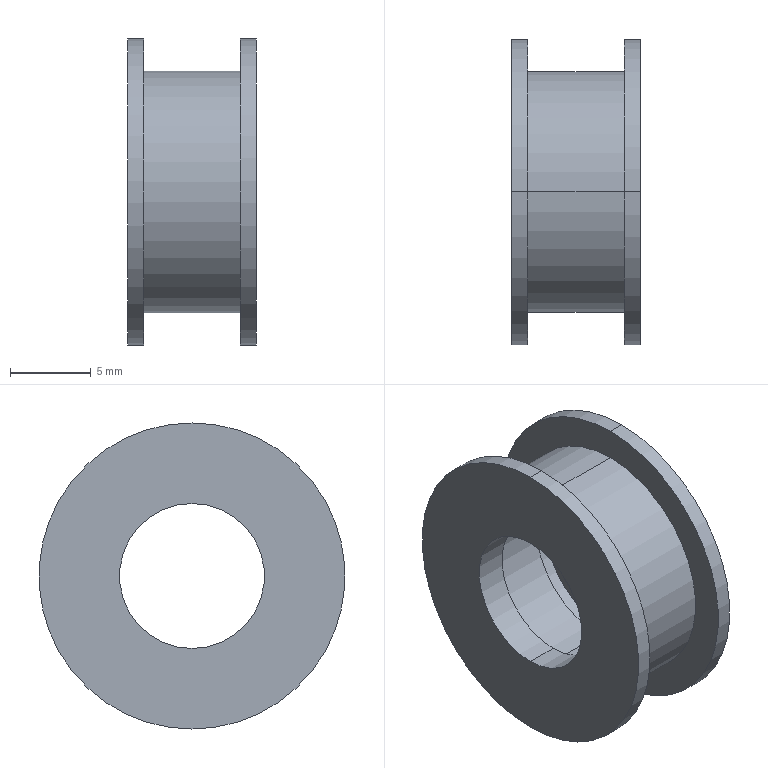Part | SolidWorks | features RefAxis 12, 3DProfileFeature 4, Revolution 1 | 1 solid | 21 faces | box 8 x 19 x 19 mm | volume 915.586 mm3 | cylinder 14 | plane 7 | commonest cylinder face diameters 11 x4 19 x4 9 x2 11.8 x2 15 x2
STEP:
#1=CARTESIAN_POINT('',(-3.,0.,9.5));
#2=VERTEX_POINT('',#1);
#3=CARTESIAN_POINT('',(-3.,0.,-9.5));
#4=VERTEX_POINT('',#3);
#5=CARTESIAN_POINT('',(-3.,0.,0.));
#6=DIRECTION('',(-1.,0.,0.));
#7=DIRECTION('',(0.,0.,1.));
#8=AXIS2_PLACEMENT_3D('',#5,#6,#7);
#9=CIRCLE('',#8,9.5);
#10=EDGE_CURVE('',#2,#4,#9,.T.);
#11=ORIENTED_EDGE('',*,*,#10,.T.);
#12=CARTESIAN_POINT('',(-4.,0.,-9.5));
#13=VERTEX_POINT('',#12);
#14=CARTESIAN_POINT('',(4.,0.,-9.5));
#15=DIRECTION('',(-1.,0.,0.));
#16=VECTOR('',#15,1000.);
#17=LINE('',#14,#16);
#18=EDGE_CURVE('',#4,#13,#17,.T.);
#19=ORIENTED_EDGE('',*,*,#18,.T.);
#20=CARTESIAN_POINT('',(-4.,0.,9.5));
#21=VERTEX_POINT('',#20);
#22=CARTESIAN_POINT('',(-4.,0.,0.));
#23=DIRECTION('',(-1.,0.,0.));
#24=DIRECTION('',(0.,0.,1.));
#25=AXIS2_PLACEMENT_3D('',#22,#23,#24);
#26=CIRCLE('',#25,9.5);
#27=EDGE_CURVE('',#21,#13,#26,.T.);
#28=ORIENTED_EDGE('',*,*,#27,.F.);
#29=CARTESIAN_POINT('',(4.,0.,9.5));
#30=DIRECTION('',(-1.,0.,0.));
#31=VECTOR('',#30,1000.);
#32=LINE('',#29,#31);
#33=EDGE_CURVE('',#2,#21,#32,.T.);
#34=ORIENTED_EDGE('',*,*,#33,.F.);
#35=EDGE_LOOP('',(#11,#19,#28,#34));
#36=FACE_OUTER_BOUND('',#35,.T.);
#37=CARTESIAN_POINT('',(4.,0.,0.));
#38=DIRECTION('',(-1.,0.,0.));
#39=DIRECTION('',(0.,0.,1.));
#40=AXIS2_PLACEMENT_3D('',#37,#38,#39);
#41=CYLINDRICAL_SURFACE('',#40,9.5);
#42=ADVANCED_FACE('',(#36),#41,.T.);
#43=CARTESIAN_POINT('',(3.,0.,7.5));
#44=VERTEX_POINT('',#43);
#45=CARTESIAN_POINT('',(3.,0.,-7.5));
#46=VERTEX_POINT('',#45);
#47=CARTESIAN_POINT('',(3.,0.,0.));
#48=DIRECTION('',(-1.,0.,0.));
#49=DIRECTION('',(0.,0.,1.));
#50=AXIS2_PLACEMENT_3D('',#47,#48,#49);
#51=CIRCLE('',#50,7.5);
#52=EDGE_CURVE('',#44,#46,#51,.T.);
#53=ORIENTED_EDGE('',*,*,#52,.T.);
#54=CARTESIAN_POINT('',(-3.,0.,-7.5));
#55=VERTEX_POINT('',#54);
#56=CARTESIAN_POINT('',(4.,0.,-7.5));
#57=DIRECTION('',(-1.,0.,0.));
#58=VECTOR('',#57,1000.);
#59=LINE('',#56,#58);
#60=EDGE_CURVE('',#46,#55,#59,.T.);
#61=ORIENTED_EDGE('',*,*,#60,.T.);
#62=CARTESIAN_POINT('',(-3.,0.,7.5));
#63=VERTEX_POINT('',#62);
#64=CARTESIAN_POINT('',(-3.,0.,0.));
#65=DIRECTION('',(-1.,0.,0.));
#66=DIRECTION('',(0.,0.,1.));
#67=AXIS2_PLACEMENT_3D('',#64,#65,#66);
#68=CIRCLE('',#67,7.5);
#69=EDGE_CURVE('',#63,#55,#68,.T.);
#70=ORIENTED_EDGE('',*,*,#69,.F.);
#71=CARTESIAN_POINT('',(4.,0.,7.5));
#72=DIRECTION('',(-1.,0.,0.));
#73=VECTOR('',#72,1000.);
#74=LINE('',#71,#73);
#75=EDGE_CURVE('',#44,#63,#74,.T.);
#76=ORIENTED_EDGE('',*,*,#75,.F.);
#77=EDGE_LOOP('',(#53,#61,#70,#76));
#78=FACE_OUTER_BOUND('',#77,.T.);
#79=CARTESIAN_POINT('',(4.,0.,0.));
#80=DIRECTION('',(-1.,0.,0.));
#81=DIRECTION('',(0.,0.,1.));
#82=AXIS2_PLACEMENT_3D('',#79,#80,#81);
#83=CYLINDRICAL_SURFACE('',#82,7.5);
#84=ADVANCED_FACE('',(#78),#83,.T.);
#85=CARTESIAN_POINT('',(4.,0.,9.5));
#86=VERTEX_POINT('',#85);
#87=CARTESIAN_POINT('',(4.,0.,-9.5));
#88=VERTEX_POINT('',#87);
#89=CARTESIAN_POINT('',(4.,0.,0.));
#90=DIRECTION('',(-1.,0.,0.));
#91=DIRECTION('',(0.,0.,1.));
#92=AXIS2_PLACEMENT_3D('',#89,#90,#91);
#93=CIRCLE('',#92,9.5);
#94=EDGE_CURVE('',#86,#88,#93,.T.);
#95=ORIENTED_EDGE('',*,*,#94,.T.);
#96=CARTESIAN_POINT('',(3.,0.,-9.5));
#97=VERTEX_POINT('',#96);
#98=CARTESIAN_POINT('',(4.,0.,-9.5));
#99=DIRECTION('',(-1.,0.,0.));
#100=VECTOR('',#99,1000.);
#101=LINE('',#98,#100);
#102=EDGE_CURVE('',#88,#97,#101,.T.);
#103=ORIENTED_EDGE('',*,*,#102,.T.);
#104=CARTESIAN_POINT('',(3.,0.,9.5));
#105=VERTEX_POINT('',#104);
#106=CARTESIAN_POINT('',(3.,0.,0.));
#107=DIRECTION('',(-1.,0.,0.));
#108=DIRECTION('',(0.,0.,1.));
#109=AXIS2_PLACEMENT_3D('',#106,#107,#108);
#110=CIRCLE('',#109,9.5);
#111=EDGE_CURVE('',#105,#97,#110,.T.);
#112=ORIENTED_EDGE('',*,*,#111,.F.);
#113=CARTESIAN_POINT('',(4.,0.,9.5));
#114=DIRECTION('',(-1.,0.,0.));
#115=VECTOR('',#114,1000.);
#116=LINE('',#113,#115);
#117=EDGE_CURVE('',#86,#105,#116,.T.);
#118=ORIENTED_EDGE('',*,*,#117,.F.);
#119=EDGE_LOOP('',(#95,#103,#112,#118));
#120=FACE_OUTER_BOUND('',#119,.T.);
#121=CARTESIAN_POINT('',(4.,0.,0.));
#122=DIRECTION('',(-1.,0.,0.));
#123=DIRECTION('',(0.,0.,1.));
#124=AXIS2_PLACEMENT_3D('',#121,#122,#123);
#125=CYLINDRICAL_SURFACE('',#124,9.5);
#126=ADVANCED_FACE('',(#120),#125,.T.);
#127=CARTESIAN_POINT('',(4.,0.,-5.5));
#128=VERTEX_POINT('',#127);
#129=CARTESIAN_POINT('',(4.,0.,5.5));
#130=VERTEX_POINT('',#129);
#131=CARTESIAN_POINT('',(4.,0.,0.));
#132=DIRECTION('',(-1.,0.,0.));
#133=DIRECTION('',(0.,0.,1.));
#134=AXIS2_PLACEMENT_3D('',#131,#132,#133);
#135=CIRCLE('',#134,5.5);
#136=EDGE_CURVE('',#128,#130,#135,.T.);
#137=ORIENTED_EDGE('',*,*,#136,.F.);
#138=CARTESIAN_POINT('',(3.,0.,-5.5));
#139=VERTEX_POINT('',#138);
#140=CARTESIAN_POINT('',(4.,0.,-5.5));
#141=DIRECTION('',(-1.,0.,0.));
#142=VECTOR('',#141,1000.);
#143=LINE('',#140,#142);
#144=EDGE_CURVE('',#128,#139,#143,.T.);
#145=ORIENTED_EDGE('',*,*,#144,.T.);
#146=CARTESIAN_POINT('',(3.,0.,5.5));
#147=VERTEX_POINT('',#146);
#148=CARTESIAN_POINT('',(3.,0.,0.));
#149=DIRECTION('',(-1.,0.,0.));
#150=DIRECTION('',(0.,0.,1.));
#151=AXIS2_PLACEMENT_3D('',#148,#149,#150);
#152=CIRCLE('',#151,5.5);
#153=EDGE_CURVE('',#139,#147,#152,.T.);
#154=ORIENTED_EDGE('',*,*,#153,.T.);
#155=CARTESIAN_POINT('',(4.,0.,5.5));
#156=DIRECTION('',(-1.,0.,0.));
#157=VECTOR('',#156,1000.);
#158=LINE('',#155,#157);
#159=EDGE_CURVE('',#130,#147,#158,.T.);
#160=ORIENTED_EDGE('',*,*,#159,.F.);
#161=EDGE_LOOP('',(#137,#145,#154,#160));
#162=FACE_OUTER_BOUND('',#161,.T.);
#163=CARTESIAN_POINT('',(4.,0.,0.));
#164=DIRECTION('',(-1.,0.,0.));
#165=DIRECTION('',(0.,0.,1.));
#166=AXIS2_PLACEMENT_3D('',#163,#164,#165);
#167=CYLINDRICAL_SURFACE('',#166,5.5);
#168=ADVANCED_FACE('',(#162),#167,.F.);
#169=CARTESIAN_POINT('',(3.,0.,-5.9));
#170=VERTEX_POINT('',#169);
#171=CARTESIAN_POINT('',(3.,0.,5.9));
#172=VERTEX_POINT('',#171);
#173=CARTESIAN_POINT('',(3.,0.,0.));
#174=DIRECTION('',(-1.,0.,0.));
#175=DIRECTION('',(0.,0.,1.));
#176=AXIS2_PLACEMENT_3D('',#173,#174,#175);
#177=CIRCLE('',#176,5.9);
#178=EDGE_CURVE('',#170,#172,#177,.T.);
#179=ORIENTED_EDGE('',*,*,#178,.F.);
#180=CARTESIAN_POINT('',(2.,0.,-5.9));
#181=VERTEX_POINT('',#180);
#182=CARTESIAN_POINT('',(4.,0.,-5.9));
#183=DIRECTION('',(-1.,0.,0.));
#184=VECTOR('',#183,1000.);
#185=LINE('',#182,#184);
#186=EDGE_CURVE('',#170,#181,#185,.T.);
#187=ORIENTED_EDGE('',*,*,#186,.T.);
#188=CARTESIAN_POINT('',(2.,0.,5.9));
#189=VERTEX_POINT('',#188);
#190=CARTESIAN_POINT('',(2.,0.,0.));
#191=DIRECTION('',(-1.,0.,0.));
#192=DIRECTION('',(0.,0.,1.));
#193=AXIS2_PLACEMENT_3D('',#190,#191,#192);
#194=CIRCLE('',#193,5.9);
#195=EDGE_CURVE('',#181,#189,#194,.T.);
#196=ORIENTED_EDGE('',*,*,#195,.T.);
#197=CARTESIAN_POINT('',(4.,0.,5.9));
#198=DIRECTION('',(-1.,0.,0.));
#199=VECTOR('',#198,1000.);
#200=LINE('',#197,#199);
#201=EDGE_CURVE('',#172,#189,#200,.T.);
#202=ORIENTED_EDGE('',*,*,#201,.F.);
#203=EDGE_LOOP('',(#179,#187,#196,#202));
#204=FACE_OUTER_BOUND('',#203,.T.);
#205=CARTESIAN_POINT('',(4.,0.,0.));
#206=DIRECTION('',(-1.,0.,0.));
#207=DIRECTION('',(0.,0.,1.));
#208=AXIS2_PLACEMENT_3D('',#205,#206,#207);
#209=CYLINDRICAL_SURFACE('',#208,5.9);
#210=ADVANCED_FACE('',(#204),#209,.F.);
#211=CARTESIAN_POINT('',(2.,0.,-5.5));
#212=VERTEX_POINT('',#211);
#213=CARTESIAN_POINT('',(2.,0.,5.5));
#214=VERTEX_POINT('',#213);
#215=CARTESIAN_POINT('',(2.,0.,0.));
#216=DIRECTION('',(-1.,0.,0.));
#217=DIRECTION('',(0.,0.,1.));
#218=AXIS2_PLACEMENT_3D('',#215,#216,#217);
#219=CIRCLE('',#218,5.5);
#220=EDGE_CURVE('',#212,#214,#219,.T.);
#221=ORIENTED_EDGE('',*,*,#220,.F.);
#222=CARTESIAN_POINT('',(-2.,0.,-5.5));
#223=VERTEX_POINT('',#222);
#224=CARTESIAN_POINT('',(4.,0.,-5.5));
#225=DIRECTION('',(-1.,0.,0.));
#226=VECTOR('',#225,1000.);
#227=LINE('',#224,#226);
#228=EDGE_CURVE('',#212,#223,#227,.T.);
#229=ORIENTED_EDGE('',*,*,#228,.T.);
#230=CARTESIAN_POINT('',(-2.,0.,5.5));
#231=VERTEX_POINT('',#230);
#232=CARTESIAN_POINT('',(-2.,0.,0.));
#233=DIRECTION('',(-1.,0.,0.));
#234=DIRECTION('',(0.,0.,1.));
#235=AXIS2_PLACEMENT_3D('',#232,#233,#234);
#236=CIRCLE('',#235,5.5);
#237=EDGE_CURVE('',#223,#231,#236,.T.);
#238=ORIENTED_EDGE('',*,*,#237,.T.);
#239=CARTESIAN_POINT('',(4.,0.,5.5));
#240=DIRECTION('',(-1.,0.,0.));
#241=VECTOR('',#240,1000.);
#242=LINE('',#239,#241);
#243=EDGE_CURVE('',#214,#231,#242,.T.);
#244=ORIENTED_EDGE('',*,*,#243,.F.);
#245=EDGE_LOOP('',(#221,#229,#238,#244));
#246=FACE_OUTER_BOUND('',#245,.T.);
#247=CARTESIAN_POINT('',(4.,0.,0.));
#248=DIRECTION('',(-1.,0.,0.));
#249=DIRECTION('',(0.,0.,1.));
#250=AXIS2_PLACEMENT_3D('',#247,#248,#249);
#251=CYLINDRICAL_SURFACE('',#250,5.5);
#252=ADVANCED_FACE('',(#246),#251,.F.);
#253=CARTESIAN_POINT('',(-2.,0.,-4.5));
#254=VERTEX_POINT('',#253);
#255=CARTESIAN_POINT('',(-2.,0.,4.5));
#256=VERTEX_POINT('',#255);
#257=CARTESIAN_POINT('',(-2.,0.,0.));
#258=DIRECTION('',(-1.,0.,0.));
#259=DIRECTION('',(0.,0.,1.));
#260=AXIS2_PLACEMENT_3D('',#257,#258,#259);
#261=CIRCLE('',#260,4.5);
#262=EDGE_CURVE('',#254,#256,#261,.T.);
#263=ORIENTED_EDGE('',*,*,#262,.F.);
#264=CARTESIAN_POINT('',(-4.,0.,-4.5));
#265=VERTEX_POINT('',#264);
#266=CARTESIAN_POINT('',(4.,0.,-4.5));
#267=DIRECTION('',(-1.,0.,0.));
#268=VECTOR('',#267,1000.);
#269=LINE('',#266,#268);
#270=EDGE_CURVE('',#254,#265,#269,.T.);
#271=ORIENTED_EDGE('',*,*,#270,.T.);
#272=CARTESIAN_POINT('',(-4.,0.,4.5));
#273=VERTEX_POINT('',#272);
#274=CARTESIAN_POINT('',(-4.,0.,0.));
#275=DIRECTION('',(-1.,0.,0.));
#276=DIRECTION('',(0.,0.,1.));
#277=AXIS2_PLACEMENT_3D('',#274,#275,#276);
#278=CIRCLE('',#277,4.5);
#279=EDGE_CURVE('',#265,#273,#278,.T.);
#280=ORIENTED_EDGE('',*,*,#279,.T.);
#281=CARTESIAN_POINT('',(4.,0.,4.5));
#282=DIRECTION('',(-1.,0.,0.));
#283=VECTOR('',#282,1000.);
#284=LINE('',#281,#283);
#285=EDGE_CURVE('',#256,#273,#284,.T.);
#286=ORIENTED_EDGE('',*,*,#285,.F.);
#287=EDGE_LOOP('',(#263,#271,#280,#286));
#288=FACE_OUTER_BOUND('',#287,.T.);
#289=CARTESIAN_POINT('',(4.,0.,0.));
#290=DIRECTION('',(-1.,0.,0.));
#291=DIRECTION('',(0.,0.,1.));
#292=AXIS2_PLACEMENT_3D('',#289,#290,#291);
#293=CYLINDRICAL_SURFACE('',#292,4.5);
#294=ADVANCED_FACE('',(#288),#293,.F.);
#295=CARTESIAN_POINT('',(-4.,0.,0.));
#296=DIRECTION('',(-1.,0.,0.));
#297=DIRECTION('',(0.,0.,1.));
#298=AXIS2_PLACEMENT_3D('',#295,#296,#297);
#299=CIRCLE('',#298,4.5);
#300=EDGE_CURVE('',#273,#265,#299,.T.);
#301=ORIENTED_EDGE('',*,*,#300,.F.);
#302=ORIENTED_EDGE('',*,*,#279,.F.);
#303=EDGE_LOOP('',(#301,#302));
#304=FACE_BOUND('',#303,.T.);
#305=ORIENTED_EDGE('',*,*,#27,.T.);
#306=CARTESIAN_POINT('',(-4.,0.,0.));
#307=DIRECTION('',(-1.,0.,0.));
#308=DIRECTION('',(0.,0.,1.));
#309=AXIS2_PLACEMENT_3D('',#306,#307,#308);
#310=CIRCLE('',#309,9.5);
#311=EDGE_CURVE('',#13,#21,#310,.T.);
#312=ORIENTED_EDGE('',*,*,#311,.T.);
#313=EDGE_LOOP('',(#305,#312));
#314=FACE_OUTER_BOUND('',#313,.T.);
#315=CARTESIAN_POINT('',(-4.,9.5,0.));
#316=DIRECTION('',(1.,0.,0.));
#317=DIRECTION('',(0.,0.,-1.));
#318=AXIS2_PLACEMENT_3D('',#315,#316,#317);
#319=PLANE('',#318);
#320=ADVANCED_FACE('',(#304,#314),#319,.F.);
#321=ORIENTED_EDGE('',*,*,#270,.F.);
#322=CARTESIAN_POINT('',(-2.,0.,0.));
#323=DIRECTION('',(-1.,0.,0.));
#324=DIRECTION('',(0.,0.,1.));
#325=AXIS2_PLACEMENT_3D('',#322,#323,#324);
#326=CIRCLE('',#325,4.5);
#327=EDGE_CURVE('',#256,#254,#326,.T.);
#328=ORIENTED_EDGE('',*,*,#327,.F.);
#329=ORIENTED_EDGE('',*,*,#285,.T.);
#330=ORIENTED_EDGE('',*,*,#300,.T.);
#331=EDGE_LOOP('',(#321,#328,#329,#330));
#332=FACE_OUTER_BOUND('',#331,.T.);
#333=CARTESIAN_POINT('',(4.,0.,0.));
#334=DIRECTION('',(-1.,0.,0.));
#335=DIRECTION('',(0.,0.,1.));
#336=AXIS2_PLACEMENT_3D('',#333,#334,#335);
#337=CYLINDRICAL_SURFACE('',#336,4.5);
#338=ADVANCED_FACE('',(#332),#337,.F.);
#339=CARTESIAN_POINT('',(-2.,0.,0.));
#340=DIRECTION('',(-1.,0.,0.));
#341=DIRECTION('',(0.,0.,1.));
#342=AXIS2_PLACEMENT_3D('',#339,#340,#341);
#343=CIRCLE('',#342,5.5);
#344=EDGE_CURVE('',#231,#223,#343,.T.);
#345=ORIENTED_EDGE('',*,*,#344,.F.);
#346=ORIENTED_EDGE('',*,*,#237,.F.);
#347=EDGE_LOOP('',(#345,#346));
#348=FACE_OUTER_BOUND('',#347,.T.);
#349=ORIENTED_EDGE('',*,*,#327,.T.);
#350=ORIENTED_EDGE('',*,*,#262,.T.);
#351=EDGE_LOOP('',(#349,#350));
#352=FACE_BOUND('',#351,.T.);
#353=CARTESIAN_POINT('',(-2.,4.5,0.));
#354=DIRECTION('',(-1.,0.,0.));
#355=DIRECTION('',(0.,0.,1.));
#356=AXIS2_PLACEMENT_3D('',#353,#354,#355);
#357=PLANE('',#356);
#358=ADVANCED_FACE('',(#348,#352),#357,.F.);
#359=ORIENTED_EDGE('',*,*,#228,.F.);
#360=CARTESIAN_POINT('',(2.,0.,0.));
#361=DIRECTION('',(-1.,0.,0.));
#362=DIRECTION('',(0.,0.,1.));
#363=AXIS2_PLACEMENT_3D('',#360,#361,#362);
#364=CIRCLE('',#363,5.5);
#365=EDGE_CURVE('',#214,#212,#364,.T.);
#366=ORIENTED_EDGE('',*,*,#365,.F.);
#367=ORIENTED_EDGE('',*,*,#243,.T.);
#368=ORIENTED_EDGE('',*,*,#344,.T.);
#369=EDGE_LOOP('',(#359,#366,#367,#368));
#370=FACE_OUTER_BOUND('',#369,.T.);
#371=CARTESIAN_POINT('',(4.,0.,0.));
#372=DIRECTION('',(-1.,0.,0.));
#373=DIRECTION('',(0.,0.,1.));
#374=AXIS2_PLACEMENT_3D('',#371,#372,#373);
#375=CYLINDRICAL_SURFACE('',#374,5.5);
#376=ADVANCED_FACE('',(#370),#375,.F.);
#377=CARTESIAN_POINT('',(2.,0.,0.));
#378=DIRECTION('',(-1.,0.,0.));
#379=DIRECTION('',(0.,0.,1.));
#380=AXIS2_PLACEMENT_3D('',#377,#378,#379);
#381=CIRCLE('',#380,5.9);
#382=EDGE_CURVE('',#189,#181,#381,.T.);
#383=ORIENTED_EDGE('',*,*,#382,.F.);
#384=ORIENTED_EDGE('',*,*,#195,.F.);
#385=EDGE_LOOP('',(#383,#384));
#386=FACE_OUTER_BOUND('',#385,.T.);
#387=ORIENTED_EDGE('',*,*,#365,.T.);
#388=ORIENTED_EDGE('',*,*,#220,.T.);
#389=EDGE_LOOP('',(#387,#388));
#390=FACE_BOUND('',#389,.T.);
#391=CARTESIAN_POINT('',(2.,5.5,0.));
#392=DIRECTION('',(-1.,0.,0.));
#393=DIRECTION('',(0.,0.,1.));
#394=AXIS2_PLACEMENT_3D('',#391,#392,#393);
#395=PLANE('',#394);
#396=ADVANCED_FACE('',(#386,#390),#395,.F.);
#397=ORIENTED_EDGE('',*,*,#186,.F.);
#398=CARTESIAN_POINT('',(3.,0.,0.));
#399=DIRECTION('',(-1.,0.,0.));
#400=DIRECTION('',(0.,0.,1.));
#401=AXIS2_PLACEMENT_3D('',#398,#399,#400);
#402=CIRCLE('',#401,5.9);
#403=EDGE_CURVE('',#172,#170,#402,.T.);
#404=ORIENTED_EDGE('',*,*,#403,.F.);
#405=ORIENTED_EDGE('',*,*,#201,.T.);
#406=ORIENTED_EDGE('',*,*,#382,.T.);
#407=EDGE_LOOP('',(#397,#404,#405,#406));
#408=FACE_OUTER_BOUND('',#407,.T.);
#409=CARTESIAN_POINT('',(4.,0.,0.));
#410=DIRECTION('',(-1.,0.,0.));
#411=DIRECTION('',(0.,0.,1.));
#412=AXIS2_PLACEMENT_3D('',#409,#410,#411);
#413=CYLINDRICAL_SURFACE('',#412,5.9);
#414=ADVANCED_FACE('',(#408),#413,.F.);
#415=CARTESIAN_POINT('',(3.,0.,0.));
#416=DIRECTION('',(-1.,0.,0.));
#417=DIRECTION('',(0.,0.,1.));
#418=AXIS2_PLACEMENT_3D('',#415,#416,#417);
#419=CIRCLE('',#418,5.5);
#420=EDGE_CURVE('',#147,#139,#419,.T.);
#421=ORIENTED_EDGE('',*,*,#420,.F.);
#422=ORIENTED_EDGE('',*,*,#153,.F.);
#423=EDGE_LOOP('',(#421,#422));
#424=FACE_BOUND('',#423,.T.);
#425=ORIENTED_EDGE('',*,*,#403,.T.);
#426=ORIENTED_EDGE('',*,*,#178,.T.);
#427=EDGE_LOOP('',(#425,#426));
#428=FACE_OUTER_BOUND('',#427,.T.);
#429=CARTESIAN_POINT('',(3.,5.9,0.));
#430=DIRECTION('',(1.,0.,0.));
#431=DIRECTION('',(0.,0.,-1.));
#432=AXIS2_PLACEMENT_3D('',#429,#430,#431);
#433=PLANE('',#432);
#434=ADVANCED_FACE('',(#424,#428),#433,.F.);
#435=ORIENTED_EDGE('',*,*,#144,.F.);
#436=CARTESIAN_POINT('',(4.,0.,0.));
#437=DIRECTION('',(-1.,0.,0.));
#438=DIRECTION('',(0.,0.,1.));
#439=AXIS2_PLACEMENT_3D('',#436,#437,#438);
#440=CIRCLE('',#439,5.5);
#441=EDGE_CURVE('',#130,#128,#440,.T.);
#442=ORIENTED_EDGE('',*,*,#441,.F.);
#443=ORIENTED_EDGE('',*,*,#159,.T.);
#444=ORIENTED_EDGE('',*,*,#420,.T.);
#445=EDGE_LOOP('',(#435,#442,#443,#444));
#446=FACE_OUTER_BOUND('',#445,.T.);
#447=CARTESIAN_POINT('',(4.,0.,0.));
#448=DIRECTION('',(-1.,0.,0.));
#449=DIRECTION('',(0.,0.,1.));
#450=AXIS2_PLACEMENT_3D('',#447,#448,#449);
#451=CYLINDRICAL_SURFACE('',#450,5.5);
#452=ADVANCED_FACE('',(#446),#451,.F.);
#453=ORIENTED_EDGE('',*,*,#94,.F.);
#454=CARTESIAN_POINT('',(4.,0.,0.));
#455=DIRECTION('',(-1.,0.,0.));
#456=DIRECTION('',(0.,0.,1.));
#457=AXIS2_PLACEMENT_3D('',#454,#455,#456);
#458=CIRCLE('',#457,9.5);
#459=EDGE_CURVE('',#88,#86,#458,.T.);
#460=ORIENTED_EDGE('',*,*,#459,.F.);
#461=EDGE_LOOP('',(#453,#460));
#462=FACE_OUTER_BOUND('',#461,.T.);
#463=ORIENTED_EDGE('',*,*,#441,.T.);
#464=ORIENTED_EDGE('',*,*,#136,.T.);
#465=EDGE_LOOP('',(#463,#464));
#466=FACE_BOUND('',#465,.T.);
#467=CARTESIAN_POINT('',(4.,5.5,0.));
#468=DIRECTION('',(-1.,0.,0.));
#469=DIRECTION('',(0.,0.,1.));
#470=AXIS2_PLACEMENT_3D('',#467,#468,#469);
#471=PLANE('',#470);
#472=ADVANCED_FACE('',(#462,#466),#471,.F.);
#473=ORIENTED_EDGE('',*,*,#102,.F.);
#474=ORIENTED_EDGE('',*,*,#459,.T.);
#475=ORIENTED_EDGE('',*,*,#117,.T.);
#476=CARTESIAN_POINT('',(3.,0.,0.));
#477=DIRECTION('',(-1.,0.,0.));
#478=DIRECTION('',(0.,0.,1.));
#479=AXIS2_PLACEMENT_3D('',#476,#477,#478);
#480=CIRCLE('',#479,9.5);
#481=EDGE_CURVE('',#97,#105,#480,.T.);
#482=ORIENTED_EDGE('',*,*,#481,.F.);
#483=EDGE_LOOP('',(#473,#474,#475,#482));
#484=FACE_OUTER_BOUND('',#483,.T.);
#485=CARTESIAN_POINT('',(4.,0.,0.));
#486=DIRECTION('',(-1.,0.,0.));
#487=DIRECTION('',(0.,0.,1.));
#488=AXIS2_PLACEMENT_3D('',#485,#486,#487);
#489=CYLINDRICAL_SURFACE('',#488,9.5);
#490=ADVANCED_FACE('',(#484),#489,.T.);
#491=ORIENTED_EDGE('',*,*,#52,.F.);
#492=CARTESIAN_POINT('',(3.,0.,0.));
#493=DIRECTION('',(-1.,0.,0.));
#494=DIRECTION('',(0.,0.,1.));
#495=AXIS2_PLACEMENT_3D('',#492,#493,#494);
#496=CIRCLE('',#495,7.5);
#497=EDGE_CURVE('',#46,#44,#496,.T.);
#498=ORIENTED_EDGE('',*,*,#497,.F.);
#499=EDGE_LOOP('',(#491,#498));
#500=FACE_BOUND('',#499,.T.);
#501=ORIENTED_EDGE('',*,*,#111,.T.);
#502=ORIENTED_EDGE('',*,*,#481,.T.);
#503=EDGE_LOOP('',(#501,#502));
#504=FACE_OUTER_BOUND('',#503,.T.);
#505=CARTESIAN_POINT('',(3.,9.5,0.));
#506=DIRECTION('',(1.,0.,0.));
#507=DIRECTION('',(0.,0.,-1.));
#508=AXIS2_PLACEMENT_3D('',#505,#506,#507);
#509=PLANE('',#508);
#510=ADVANCED_FACE('',(#500,#504),#509,.F.);
#511=ORIENTED_EDGE('',*,*,#60,.F.);
#512=ORIENTED_EDGE('',*,*,#497,.T.);
#513=ORIENTED_EDGE('',*,*,#75,.T.);
#514=CARTESIAN_POINT('',(-3.,0.,0.));
#515=DIRECTION('',(-1.,0.,0.));
#516=DIRECTION('',(0.,0.,1.));
#517=AXIS2_PLACEMENT_3D('',#514,#515,#516);
#518=CIRCLE('',#517,7.5);
#519=EDGE_CURVE('',#55,#63,#518,.T.);
#520=ORIENTED_EDGE('',*,*,#519,.F.);
#521=EDGE_LOOP('',(#511,#512,#513,#520));
#522=FACE_OUTER_BOUND('',#521,.T.);
#523=CARTESIAN_POINT('',(4.,0.,0.));
#524=DIRECTION('',(-1.,0.,0.));
#525=DIRECTION('',(0.,0.,1.));
#526=AXIS2_PLACEMENT_3D('',#523,#524,#525);
#527=CYLINDRICAL_SURFACE('',#526,7.5);
#528=ADVANCED_FACE('',(#522),#527,.T.);
#529=ORIENTED_EDGE('',*,*,#10,.F.);
#530=CARTESIAN_POINT('',(-3.,0.,0.));
#531=DIRECTION('',(-1.,0.,0.));
#532=DIRECTION('',(0.,0.,1.));
#533=AXIS2_PLACEMENT_3D('',#530,#531,#532);
#534=CIRCLE('',#533,9.5);
#535=EDGE_CURVE('',#4,#2,#534,.T.);
#536=ORIENTED_EDGE('',*,*,#535,.F.);
#537=EDGE_LOOP('',(#529,#536));
#538=FACE_OUTER_BOUND('',#537,.T.);
#539=ORIENTED_EDGE('',*,*,#69,.T.);
#540=ORIENTED_EDGE('',*,*,#519,.T.);
#541=EDGE_LOOP('',(#539,#540));
#542=FACE_BOUND('',#541,.T.);
#543=CARTESIAN_POINT('',(-3.,7.5,0.));
#544=DIRECTION('',(-1.,0.,0.));
#545=DIRECTION('',(0.,0.,1.));
#546=AXIS2_PLACEMENT_3D('',#543,#544,#545);
#547=PLANE('',#546);
#548=ADVANCED_FACE('',(#538,#542),#547,.F.);
#549=ORIENTED_EDGE('',*,*,#18,.F.);
#550=ORIENTED_EDGE('',*,*,#535,.T.);
#551=ORIENTED_EDGE('',*,*,#33,.T.);
#552=ORIENTED_EDGE('',*,*,#311,.F.);
#553=EDGE_LOOP('',(#549,#550,#551,#552));
#554=FACE_OUTER_BOUND('',#553,.T.);
#555=CARTESIAN_POINT('',(4.,0.,0.));
#556=DIRECTION('',(-1.,0.,0.));
#557=DIRECTION('',(0.,0.,1.));
#558=AXIS2_PLACEMENT_3D('',#555,#556,#557);
#559=CYLINDRICAL_SURFACE('',#558,9.5);
#560=ADVANCED_FACE('',(#554),#559,.T.);
#561=CLOSED_SHELL('',(#42,#84,#126,#168,#210,#252,#294,#320,#338,#358,#376,#396,#414,#434,#452,#472,#490,#510,#528,#548,#560));
#562=MANIFOLD_SOLID_BREP('',#561);
#563=CARTESIAN_POINT('',(0.,0.,0.));
#564=DIRECTION('',(0.,0.,1.));
#565=DIRECTION('',(1.,0.,0.));
#566=AXIS2_PLACEMENT_3D('',#563,#564,#565);
#567=(LENGTH_UNIT()NAMED_UNIT(*)SI_UNIT(.MILLI.,.METRE.));
#568=UNCERTAINTY_MEASURE_WITH_UNIT(LENGTH_MEASURE(0.00001),#567,'','');
#569=(NAMED_UNIT(*)PLANE_ANGLE_UNIT()SI_UNIT($,.RADIAN.));
#570=(NAMED_UNIT(*)SI_UNIT($,.STERADIAN.)SOLID_ANGLE_UNIT());
#571=(GEOMETRIC_REPRESENTATION_CONTEXT(3)GLOBAL_UNCERTAINTY_ASSIGNED_CONTEXT((#568))GLOBAL_UNIT_ASSIGNED_CONTEXT((#567,#569,#570))REPRESENTATION_CONTEXT('',''));
#572=ADVANCED_BREP_SHAPE_REPRESENTATION('',(#562,#566),#571);